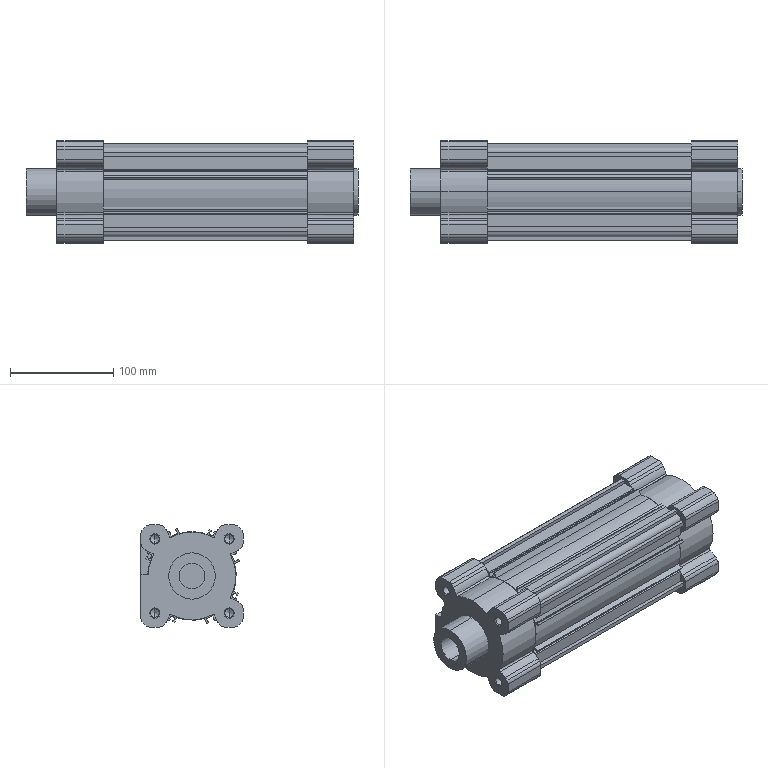Part | SolidWorks | features BaseBody 1 | 1 solid | 310 faces | box 322 x 99 x 99 mm | volume 1340273 mm3 | plane 140 | cylinder 130 | cone 40 | commonest cylinder face diameters 10 x30 3 x18 8.376 x16 28 x14 85.2 x10 4.25 x9